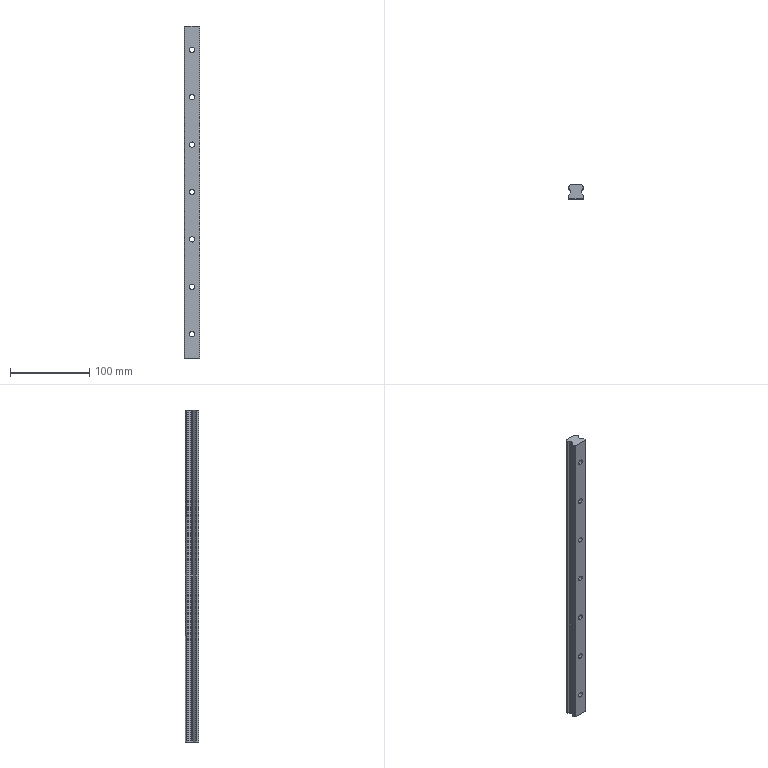Part | STEP file | HGR20_3_AF0_1 | 1 solid | 79 faces | box 20 x 17.5 x 420 mm | volume 118454 mm3 | cylinder 50 | plane 29 | commonest cylinder face diameters 6.6 x14 11 x14 1 x12 2 x6 4.06 x4